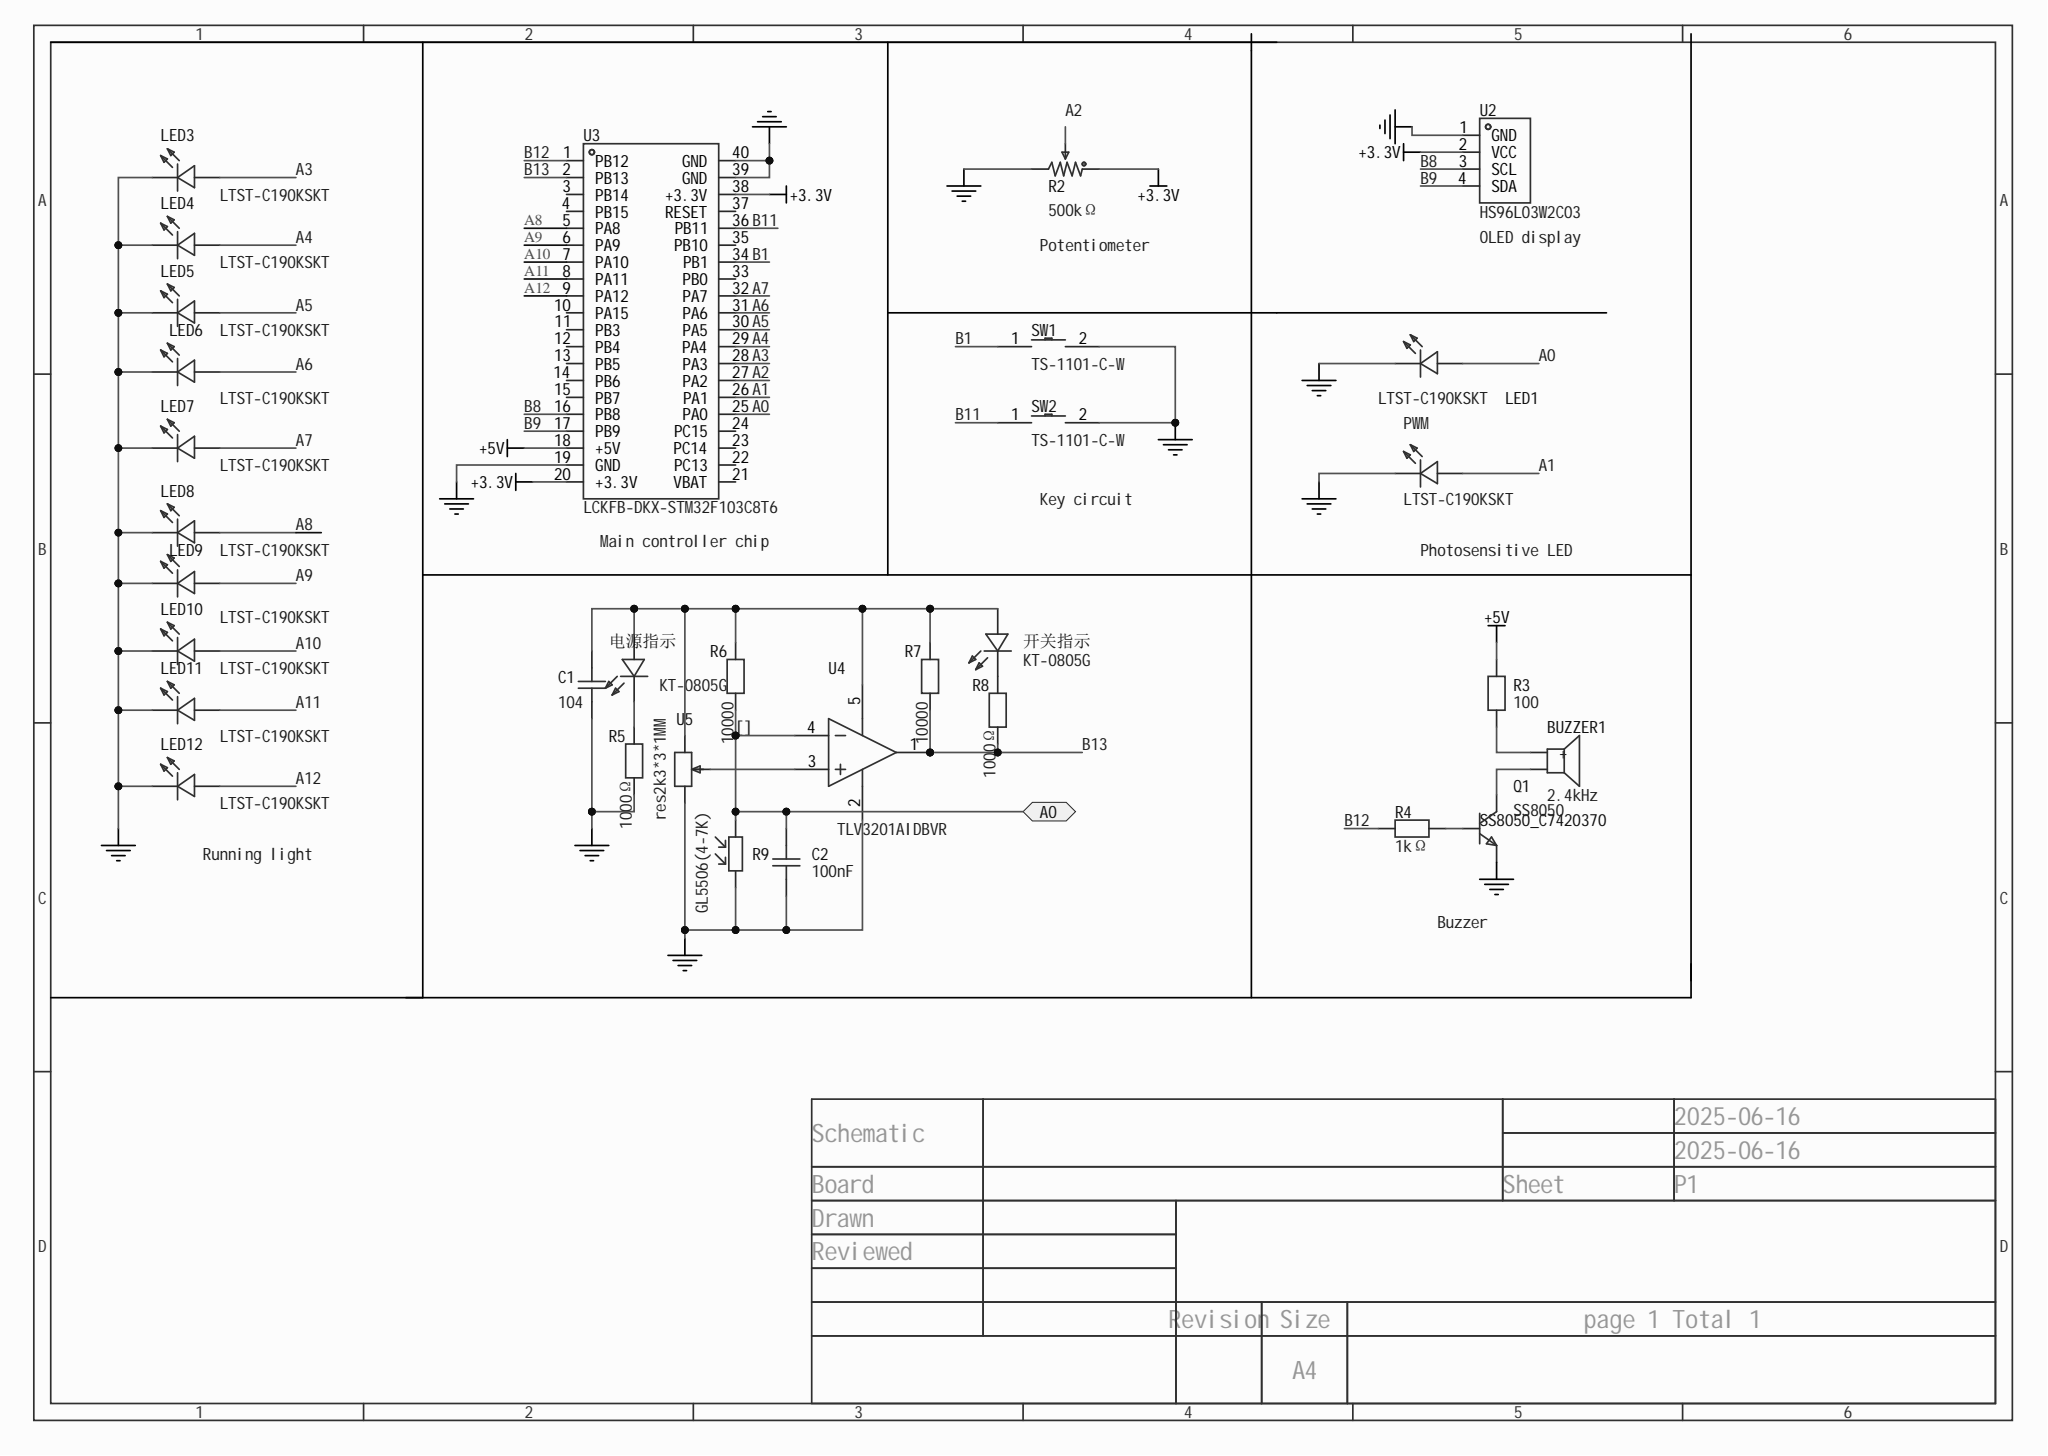Circuit board | Altium Designer | 32 parts | 29 nets
Bill of materials:
Comment,Description,Designator,Footprint,LibRef,Quantity
"2.4kHz","","BUZZER1","BUZZER","TMB12A05_C96093","1"
"104","","C1","RAD-0.1","0603F104Z500CT_C83060","1"
"100nF","","C2","RAD-0.1","0603F104Z500CT_C83060","1"
"LTST-C190KSKT","","LED1, LED2, LED3, LED4, LED5, LED6, LED7, LED8, LED9, LED10, LED11, LED12","LED3MM","LTST-C190KSKT","12"
"SS8050","","Q1","TO-92","SS8050_C7420370","1"
"500kΩ","","R2","3296W","3362W-1-504LF","1"
"100","","R3","RS 1/4W","RE1206F1R050","1"
"1kΩ","","R4","RS 1/4W","FCR0603F1K","1"
"1000Ω","","R5, R8","RS 1/4W","HVLR2505F1G00K9","2"
"10000","","R6, R7","RS 1/4W","HVLR2505F1G00K9","2"
"GL5506(4-7K)","","R9","RS 1/4W","GL5506（4-7K）","1"
"TS-1101-C-W","","SW1, SW2","四脚轻触开关","TS-1101-C-W","2"
"HS96L03W2C03","","U2","0.96OLED_4P","HS96L03W2C03","1"
"LCKFB-DKX-STM32F103C8T6","","U3","STM32核心板","LCKFB-DKX-STM32F103C8T6","1"
"TLV3201AIDBVR","","U4","SOT-23-5_L3.0-W1.7-P0.95-LS2.8-BR","TLV3201AIDBVR","1"
"res2k3*3*1MM","","U5","3296W","res2k3*3*1MM","1"
"KT-0805G","","开关指示, 电源指示","LED3MM","KT-0805G","2"
Netlist (Protel format):
[
BUZZER1
BUZZER
2.4kHz



]
[
C1
RAD-0.1
104



]
[
C2
RAD-0.1
100nF



]
[
LED1
LED3MM
LTST-C190KSKT



]
[
LED2
LED3MM
LTST-C190KSKT



]
[
LED3
LED3MM
LTST-C190KSKT



]
[
LED4
LED3MM
LTST-C190KSKT



]
[
LED5
LED3MM
LTST-C190KSKT



]
[
LED6
LED3MM
LTST-C190KSKT



]
[
LED7
LED3MM
LTST-C190KSKT



]
[
LED8
LED3MM
LTST-C190KSKT



]
[
LED9
LED3MM
LTST-C190KSKT



]
[
LED10
LED3MM
LTST-C190KSKT



]
[
LED11
LED3MM
LTST-C190KSKT



]
[
LED12
LED3MM
LTST-C190KSKT



]
[
Q1
TO-92
SS8050



]
[
R2
3296W
500kΩ



]
[
R3
RS 1/4W
100



]
[
R4
RS 1/4W
1kΩ



]
[
R5
RS 1/4W
1000Ω



]
[
R6
RS 1/4W
10000



]
[
R7
RS 1/4W
10000



]
[
R8
RS 1/4W
1000Ω



]
[
R9
RS 1/4W
GL5506(4-7K)



]
[
SW1
四脚轻触开关
TS-1101-C-W



]
[
SW2
四脚轻触开关
TS-1101-C-W



]
[
U2
0.96OLED_4P
HS96L03W2C03



]
[
U3
STM32核心板
LCKFB-DKX-STM32F103C8T6



]
[
U4
SOT-23-5_L3.0-W1.7-P0.95-LS2.8-BR
TLV3201AIDBVR



]
[
U5
3296W
res2k3*3*1MM



]
[
开关指示
LED3MM
KT-0805G



]
[
电源指示
LED3MM
KT-0805G



]
(
NetU4_3
U4-3
U5-2
)
(
NetR8_2
R8-2
开关指示-2
)
(
NetR5_2
R5-2
电源指示-2
)
(
NetQ1_1
Q1-1
R4-2
)
(
NetC1_2
C1-2
R6-2
R7-2
U4-5
U5-3
开关指示-1
电源指示-1
)
(
NetBUZZER1_2
BUZZER1-2
Q1-3
)
(
NetBUZZER1_1
BUZZER1-1
R3-1
)
(
GND
C1-1
C2-1
LED1-1
LED2-1
LED3-1
LED4-1
LED5-1
LED6-1
LED7-1
LED8-1
LED9-1
LED10-1
LED11-1
LED12-1
Q1-2
R2-3
R5-1
R9-2
SW1-2
SW2-2
U2-1
U3-19
U3-39
U3-40
U4-2
U5-1
)
(
B13
R7-1
R8-1
U3-2
U4-1
)
(
B12
R4-1
U3-1
)
(
B11
SW2-1
U3-36
)
(
B9
U2-4
U3-17
)
(
B8
U2-3
U3-16
)
(
B1
SW1-1
U3-34
)
(
A12
LED12-2
U3-9
)
(
A11
LED11-2
U3-8
)
(
A10
LED10-2
U3-7
)
(
A9
LED9-2
U3-6
)
(
A8
LED8-2
U3-5
)
(
A7
LED7-2
U3-32
)
(
A6
LED6-2
U3-31
)
(
A5
LED5-2
U3-30
)
(
A4
LED4-2
U3-29
)
(
A3
LED3-2
U3-28
)
(
A1
LED2-2
U3-26
)
(
A0
LED1-2
U3-25
)
(
[]
C2-2
R6-1
R9-1
U4-4
)
(
+5V
R3-2
U3-18
)
(
+3.3V
R2-1
U2-2
U3-20
U3-38
)